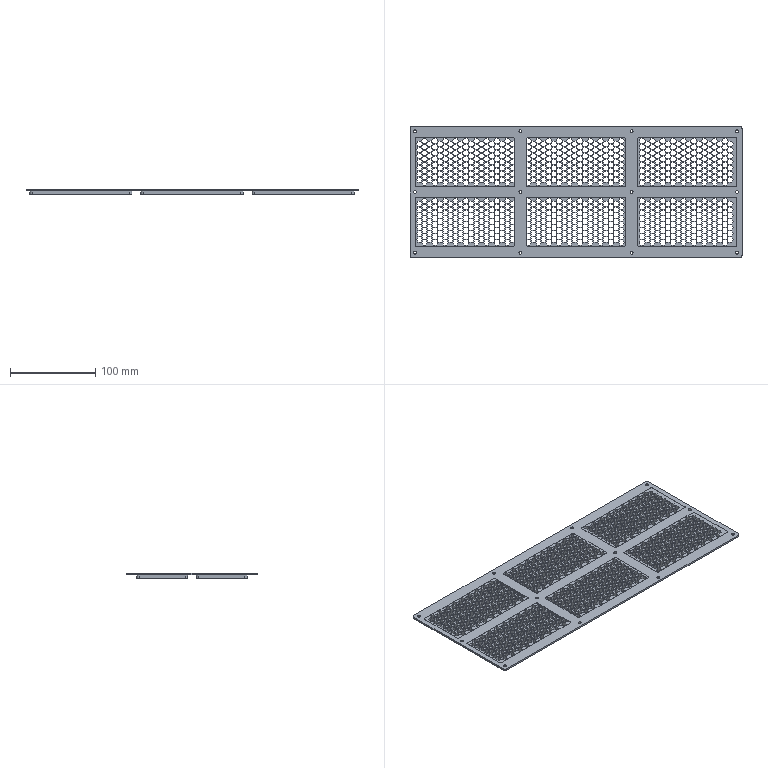NC program | NX | posted with a generic post
Lines 1 to 1112 of 172913:
N10 G17 G21 G94 G90
(PLANAR_MILL_3 , TOOL : D6_FINISH)
N12 T02 M6
N14 G54
N16 G17 G0 G90 X0. Y-79.75 S6500 M3
N18 G43 Z20. H2
N20 Z6.009
N22 G94 G1 Z3.009 F2000.
N24 Y-76.75
N26 X-191.5
N28 G2 X-194.25 Y-74. R2.75
N30 G1 Y74.
N32 G2 X-191.5 Y76.75 R2.75
N34 G1 X191.5
N36 G2 X194.25 Y74. R2.75
N38 G1 Y-74.
N40 G2 X191.5 Y-76.75 R2.75
N42 G1 X0.
N44 Y-71.95
N46 X-189.45
N48 Y-68.408
N50 G3 X-187. Y-68.86 R6.86
N52 G1 X-73.
N54 G3 X-66.659 Y-64.617 R6.86
N56 G1 X-62.222 Y-66.449
N58 G3 X-61.532 Y-67.15 R6.86
N60 G1 X-62.539
N62 X-65.437 Y-68.712
N64 X-62.539 Y-67.15
N66 G3 X-62.222 Y-66.449 R11.66
N68 G1 X-66.659 Y-64.617
N70 G3 X-66.14 Y-62. R6.86
N72 G1 Y-8.
N74 G3 X-73. Y-1.14 R6.86
N76 G1 X-187.
N78 G3 X-189.45 Y-1.592 R6.86
N80 G1 X-189.107 Y-2.489
N82 G2 X-187. Y-2.1 R5.9
N84 G1 X-73.
N86 G2 X-67.1 Y-8. R5.9
N88 G1 Y-62.
N90 G2 X-73. Y-67.9 R5.9
N92 G1 X-187.
N94 G2 X-192.9 Y-62. R5.9
N96 G1 Y-8.
N98 G2 X-189.107 Y-2.489 R5.9
N100 G1 X-189.45 Y-1.592
N102 Y1.592
N104 G3 X-187. Y1.14 R6.86
N106 G1 X-73.
N108 G3 X-66.14 Y8. R6.86
N110 G1 Y62.
N112 G3 X-73. Y68.86 R6.86
N114 G1 X-187.
N116 G3 X-189.45 Y68.408 R6.86
N118 G1 X-189.107 Y67.511
N120 G2 X-187. Y67.9 R5.9
N122 G1 X-73.
N124 G2 X-67.1 Y62. R5.9
N126 G1 Y8.
N128 G2 X-73. Y2.1 R5.9
N130 G1 X-187.
N132 G2 X-192.9 Y8. R5.9
N134 G1 Y62.
N136 G2 X-189.107 Y67.511 R5.9
N138 G1 X-189.45 Y68.408
N140 Y71.95
N142 X-61.532
N144 Y67.15
N146 G3 X-62.222 Y66.449 R6.86
N148 X-62.539 Y67.15 R11.66
N150 G1 X-65.437 Y68.712
N152 X-62.539 Y67.15
N154 X-61.532
N156 Y71.95
N158 X189.45
N160 Y68.408
N162 G3 X187. Y68.86 R6.86
N164 G1 X73.
N166 G3 X66.659 Y64.617 R6.86
N168 G1 X62.222 Y66.449
N170 G3 X61.532 Y67.15 R6.86
N172 G1 X59.132 Y68.95
N174 X-59.132
N176 G2 X-58.901 Y68.591 R3.
N178 X-57. Y68.86 R6.86
N180 G1 X57.
N182 G2 X58.901 Y68.591 R6.86
N184 X59.132 Y68.95 R3.
N186 G1 X61.532 Y67.15
N188 X62.539
N190 X65.437 Y68.712
N192 X62.539 Y67.15
N194 G3 X62.222 Y66.449 R11.66
N196 G1 X66.659 Y64.617
N198 G3 X66.14 Y62. R6.86
N200 G1 Y8.
N202 G3 X73. Y1.14 R6.86
N204 G1 X187.
N206 G3 X189.45 Y1.592 R6.86
N208 G1 X189.107 Y2.489
N210 G2 X187. Y2.1 R5.9
N212 G1 X73.
N214 G2 X67.1 Y8. R5.9
N216 G1 Y62.
N218 G2 X73. Y67.9 R5.9
N220 G1 X187.
N222 G2 X192.9 Y62. R5.9
N224 G1 Y8.
N226 G2 X189.107 Y2.489 R5.9
N228 G1 X189.45 Y1.592
N230 Y-1.592
N232 G3 X187. Y-1.14 R6.86
N234 G1 X73.
N236 G3 X66.659 Y-5.383 R6.86
N238 G1 X62.222 Y-3.551
N240 G3 X57. Y-1.14 R6.86
N242 G1 X-57.
N244 G3 X-62.222 Y-3.551 R6.86
N246 X-64.517 Y0. R11.66
N248 X-62.222 Y3.551 R11.66
N250 X-57. Y1.14 R6.86
N252 G1 X57.
N254 G3 X62.222 Y3.551 R6.86
N256 G1 X61.491 Y4.174
N258 G2 X57. Y2.1 R5.9
N260 G1 X-57.
N262 G2 X-62.9 Y8. R5.9
N264 G1 Y62.
N266 G2 X-57. Y67.9 R5.9
N268 G1 X57.
N270 G2 X62.9 Y62. R5.9
N272 G1 Y8.
N274 G2 X61.491 Y4.174 R5.9
N276 G1 X62.222 Y3.551
N278 G3 X64.517 Y0. R11.66
N280 X62.222 Y-3.551 R11.66
N282 G1 X66.659 Y-5.383
N284 G3 X66.14 Y-8. R6.86
N286 G1 Y-62.
N288 G3 X73. Y-68.86 R6.86
N290 G1 X187.
N292 G3 X189.45 Y-68.408 R6.86
N294 G1 X189.107 Y-67.511
N296 G2 X187. Y-67.9 R5.9
N298 G1 X73.
N300 G2 X67.1 Y-62. R5.9
N302 G1 Y-8.
N304 G2 X73. Y-2.1 R5.9
N306 G1 X187.
N308 G2 X192.9 Y-8. R5.9
N310 G1 Y-62.
N312 G2 X189.107 Y-67.511 R5.9
N314 G1 X189.45 Y-68.408
N316 Y-71.95
N318 X61.532
N320 Y-67.15
N322 G3 X62.222 Y-66.449 R6.86
N324 G1 X61.491 Y-65.826
N326 G2 X57. Y-67.9 R5.9
N328 G1 X-57.
N330 G2 X-62.9 Y-62. R5.9
N332 G1 Y-8.
N334 G2 X-57. Y-2.1 R5.9
N336 G1 X57.
N338 G2 X62.9 Y-8. R5.9
N340 G1 Y-62.
N342 G2 X61.491 Y-65.826 R5.9
N344 G1 X62.222 Y-66.449
N346 G3 X62.539 Y-67.15 R11.66
N348 G1 X65.437 Y-68.712
N350 X62.539 Y-67.15
N352 X61.532
N354 X58.901 Y-68.591
N356 G2 X57. Y-68.86 R6.86
N358 G1 X-57.
N360 G2 X-58.901 Y-68.591 R6.86
N362 X-59.132 Y-68.95 R3.
N364 G1 X59.132
N366 G2 X58.901 Y-68.591 R3.
N368 G1 X61.532 Y-67.15
N370 Y-71.95
N372 X0.
N374 Y-74.95
N376 Z6.009
N378 G0 Z20.
N380 Y-79.75
N382 Z5.519
N384 G1 Z2.519
N386 Y-76.75
N388 X-191.5
N390 G2 X-194.25 Y-74. R2.75
N392 G1 Y74.
N394 G2 X-191.5 Y76.75 R2.75
N396 G1 X191.5
N398 G2 X194.25 Y74. R2.75
N400 G1 Y-74.
N402 G2 X191.5 Y-76.75 R2.75
N404 G1 X0.
N406 Y-71.95
N408 X-189.45
N410 Y-68.408
N412 G3 X-187. Y-68.86 R6.86
N414 G1 X-73.
N416 G3 X-66.659 Y-64.617 R6.86
N418 G1 X-62.222 Y-66.449
N420 G3 X-61.532 Y-67.15 R6.86
N422 G1 X-62.539
N424 X-65.437 Y-68.712
N426 X-62.539 Y-67.15
N428 G3 X-62.222 Y-66.449 R11.66
N430 G1 X-66.659 Y-64.617
N432 G3 X-66.14 Y-62. R6.86
N434 G1 Y-8.
N436 G3 X-73. Y-1.14 R6.86
N438 G1 X-187.
N440 G3 X-189.45 Y-1.592 R6.86
N442 G1 X-189.107 Y-2.489
N444 G2 X-187. Y-2.1 R5.9
N446 G1 X-73.
N448 G2 X-67.1 Y-8. R5.9
N450 G1 Y-62.
N452 G2 X-73. Y-67.9 R5.9
N454 G1 X-187.
N456 G2 X-192.9 Y-62. R5.9
N458 G1 Y-8.
N460 G2 X-189.107 Y-2.489 R5.9
N462 G1 X-189.45 Y-1.592
N464 Y1.592
N466 G3 X-187. Y1.14 R6.86
N468 G1 X-73.
N470 G3 X-66.14 Y8. R6.86
N472 G1 Y62.
N474 G3 X-73. Y68.86 R6.86
N476 G1 X-187.
N478 G3 X-189.45 Y68.408 R6.86
N480 G1 X-189.107 Y67.511
N482 G2 X-187. Y67.9 R5.9
N484 G1 X-73.
N486 G2 X-67.1 Y62. R5.9
N488 G1 Y8.
N490 G2 X-73. Y2.1 R5.9
N492 G1 X-187.
N494 G2 X-192.9 Y8. R5.9
N496 G1 Y62.
N498 G2 X-189.107 Y67.511 R5.9
N500 G1 X-189.45 Y68.408
N502 Y71.95
N504 X-61.532
N506 Y67.15
N508 G3 X-62.222 Y66.449 R6.86
N510 X-62.539 Y67.15 R11.66
N512 G1 X-65.437 Y68.712
N514 X-62.539 Y67.15
N516 X-61.532
N518 Y71.95
N520 X189.45
N522 Y68.408
N524 G3 X187. Y68.86 R6.86
N526 G1 X73.
N528 G3 X66.659 Y64.617 R6.86
N530 G1 X62.222 Y66.449
N532 G3 X61.532 Y67.15 R6.86
N534 G1 X59.132 Y68.95
N536 X-59.132
N538 G2 X-58.901 Y68.591 R3.
N540 X-57. Y68.86 R6.86
N542 G1 X57.
N544 G2 X58.901 Y68.591 R6.86
N546 X59.132 Y68.95 R3.
N548 G1 X61.532 Y67.15
N550 X62.539
N552 X65.437 Y68.712
N554 X62.539 Y67.15
N556 G3 X62.222 Y66.449 R11.66
N558 G1 X66.659 Y64.617
N560 G3 X66.14 Y62. R6.86
N562 G1 Y8.
N564 G3 X73. Y1.14 R6.86
N566 G1 X187.
N568 G3 X189.45 Y1.592 R6.86
N570 G1 X189.107 Y2.489
N572 G2 X187. Y2.1 R5.9
N574 G1 X73.
N576 G2 X67.1 Y8. R5.9
N578 G1 Y62.
N580 G2 X73. Y67.9 R5.9
N582 G1 X187.
N584 G2 X192.9 Y62. R5.9
N586 G1 Y8.
N588 G2 X189.107 Y2.489 R5.9
N590 G1 X189.45 Y1.592
N592 Y-1.592
N594 G3 X187. Y-1.14 R6.86
N596 G1 X73.
N598 G3 X66.659 Y-5.383 R6.86
N600 G1 X62.222 Y-3.551
N602 G3 X57. Y-1.14 R6.86
N604 G1 X-57.
N606 G3 X-62.222 Y-3.551 R6.86
N608 X-64.517 Y0. R11.66
N610 X-62.222 Y3.551 R11.66
N612 X-57. Y1.14 R6.86
N614 G1 X57.
N616 G3 X62.222 Y3.551 R6.86
N618 G1 X61.491 Y4.174
N620 G2 X57. Y2.1 R5.9
N622 G1 X-57.
N624 G2 X-62.9 Y8. R5.9
N626 G1 Y62.
N628 G2 X-57. Y67.9 R5.9
N630 G1 X57.
N632 G2 X62.9 Y62. R5.9
N634 G1 Y8.
N636 G2 X61.491 Y4.174 R5.9
N638 G1 X62.222 Y3.551
N640 G3 X64.517 Y0. R11.66
N642 X62.222 Y-3.551 R11.66
N644 G1 X66.659 Y-5.383
N646 G3 X66.14 Y-8. R6.86
N648 G1 Y-62.
N650 G3 X73. Y-68.86 R6.86
N652 G1 X187.
N654 G3 X189.45 Y-68.408 R6.86
N656 G1 X189.107 Y-67.511
N658 G2 X187. Y-67.9 R5.9
N660 G1 X73.
N662 G2 X67.1 Y-62. R5.9
N664 G1 Y-8.
N666 G2 X73. Y-2.1 R5.9
N668 G1 X187.
N670 G2 X192.9 Y-8. R5.9
N672 G1 Y-62.
N674 G2 X189.107 Y-67.511 R5.9
N676 G1 X189.45 Y-68.408
N678 Y-71.95
N680 X61.532
N682 Y-67.15
N684 G3 X62.222 Y-66.449 R6.86
N686 G1 X61.491 Y-65.826
N688 G2 X57. Y-67.9 R5.9
N690 G1 X-57.
N692 G2 X-62.9 Y-62. R5.9
N694 G1 Y-8.
N696 G2 X-57. Y-2.1 R5.9
N698 G1 X57.
N700 G2 X62.9 Y-8. R5.9
N702 G1 Y-62.
N704 G2 X61.491 Y-65.826 R5.9
N706 G1 X62.222 Y-66.449
N708 G3 X62.539 Y-67.15 R11.66
N710 G1 X65.437 Y-68.712
N712 X62.539 Y-67.15
N714 X61.532
N716 X58.901 Y-68.591
N718 G2 X57. Y-68.86 R6.86
N720 G1 X-57.
N722 G2 X-58.901 Y-68.591 R6.86
N724 X-59.132 Y-68.95 R3.
N726 G1 X59.132
N728 G2 X58.901 Y-68.591 R3.
N730 G1 X61.532 Y-67.15
N732 Y-71.95
N734 X0.
N736 Y-74.95
N738 Z5.519
N740 G0 Z20.
N742 Y-79.75
N744 Z5.028
N746 G1 Z2.028
N748 Y-76.75
N750 X-191.5
N752 G2 X-194.25 Y-74. R2.75
N754 G1 Y74.
N756 G2 X-191.5 Y76.75 R2.75
N758 G1 X191.5
N760 G2 X194.25 Y74. R2.75
N762 G1 Y-74.
N764 G2 X191.5 Y-76.75 R2.75
N766 G1 X0.
N768 Y-71.95
N770 X-189.45
N772 Y-68.408
N774 G3 X-187. Y-68.86 R6.86
N776 G1 X-73.
N778 G3 X-66.659 Y-64.617 R6.86
N780 G1 X-62.222 Y-66.449
N782 G3 X-61.532 Y-67.15 R6.86
N784 G1 X-62.539
N786 X-65.437 Y-68.712
N788 X-62.539 Y-67.15
N790 G3 X-62.222 Y-66.449 R11.66
N792 G1 X-66.659 Y-64.617
N794 G3 X-66.14 Y-62. R6.86
N796 G1 Y-8.
N798 G3 X-73. Y-1.14 R6.86
N800 G1 X-187.
N802 G3 X-189.45 Y-1.592 R6.86
N804 G1 X-189.107 Y-2.489
N806 G2 X-187. Y-2.1 R5.9
N808 G1 X-73.
N810 G2 X-67.1 Y-8. R5.9
N812 G1 Y-62.
N814 G2 X-73. Y-67.9 R5.9
N816 G1 X-187.
N818 G2 X-192.9 Y-62. R5.9
N820 G1 Y-8.
N822 G2 X-189.107 Y-2.489 R5.9
N824 G1 X-189.45 Y-1.592
N826 Y1.592
N828 G3 X-187. Y1.14 R6.86
N830 G1 X-73.
N832 G3 X-66.14 Y8. R6.86
N834 G1 Y62.
N836 G3 X-73. Y68.86 R6.86
N838 G1 X-187.
N840 G3 X-189.45 Y68.408 R6.86
N842 G1 X-189.107 Y67.511
N844 G2 X-187. Y67.9 R5.9
N846 G1 X-73.
N848 G2 X-67.1 Y62. R5.9
N850 G1 Y8.
N852 G2 X-73. Y2.1 R5.9
N854 G1 X-187.
N856 G2 X-192.9 Y8. R5.9
N858 G1 Y62.
N860 G2 X-189.107 Y67.511 R5.9
N862 G1 X-189.45 Y68.408
N864 Y71.95
N866 X-61.532
N868 Y67.15
N870 G3 X-62.222 Y66.449 R6.86
N872 X-62.539 Y67.15 R11.66
N874 G1 X-65.437 Y68.712
N876 X-62.539 Y67.15
N878 X-61.532
N880 Y71.95
N882 X189.45
N884 Y68.408
N886 G3 X187. Y68.86 R6.86
N888 G1 X73.
N890 G3 X66.659 Y64.617 R6.86
N892 G1 X62.222 Y66.449
N894 G3 X61.532 Y67.15 R6.86
N896 G1 X59.132 Y68.95
N898 X-59.132
N900 G2 X-58.901 Y68.591 R3.
N902 X-57. Y68.86 R6.86
N904 G1 X57.
N906 G2 X58.901 Y68.591 R6.86
N908 X59.132 Y68.95 R3.
N910 G1 X61.532 Y67.15
N912 X62.539
N914 X65.437 Y68.712
N916 X62.539 Y67.15
N918 G3 X62.222 Y66.449 R11.66
N920 G1 X66.659 Y64.617
N922 G3 X66.14 Y62. R6.86
N924 G1 Y8.
N926 G3 X73. Y1.14 R6.86
N928 G1 X187.
N930 G3 X189.45 Y1.592 R6.86
N932 G1 X189.107 Y2.489
N934 G2 X187. Y2.1 R5.9
N936 G1 X73.
N938 G2 X67.1 Y8. R5.9
N940 G1 Y62.
N942 G2 X73. Y67.9 R5.9
N944 G1 X187.
N946 G2 X192.9 Y62. R5.9
N948 G1 Y8.
N950 G2 X189.107 Y2.489 R5.9
N952 G1 X189.45 Y1.592
N954 Y-1.592
N956 G3 X187. Y-1.14 R6.86
N958 G1 X73.
N960 G3 X66.659 Y-5.383 R6.86
N962 G1 X62.222 Y-3.551
N964 G3 X57. Y-1.14 R6.86
N966 G1 X-57.
N968 G3 X-62.222 Y-3.551 R6.86
N970 X-64.517 Y0. R11.66
N972 X-62.222 Y3.551 R11.66
N974 X-57. Y1.14 R6.86
N976 G1 X57.
N978 G3 X62.222 Y3.551 R6.86
N980 G1 X61.491 Y4.174
N982 G2 X57. Y2.1 R5.9
N984 G1 X-57.
N986 G2 X-62.9 Y8. R5.9
N988 G1 Y62.
N990 G2 X-57. Y67.9 R5.9
N992 G1 X57.
N994 G2 X62.9 Y62. R5.9
N996 G1 Y8.
N998 G2 X61.491 Y4.174 R5.9
N1000 G1 X62.222 Y3.551
N1002 G3 X64.517 Y0. R11.66
N1004 X62.222 Y-3.551 R11.66
N1006 G1 X66.659 Y-5.383
N1008 G3 X66.14 Y-8. R6.86
N1010 G1 Y-62.
N1012 G3 X73. Y-68.86 R6.86
N1014 G1 X187.
N1016 G3 X189.45 Y-68.408 R6.86
N1018 G1 X189.107 Y-67.511
N1020 G2 X187. Y-67.9 R5.9
N1022 G1 X73.
N1024 G2 X67.1 Y-62. R5.9
N1026 G1 Y-8.
N1028 G2 X73. Y-2.1 R5.9
N1030 G1 X187.
N1032 G2 X192.9 Y-8. R5.9
N1034 G1 Y-62.
N1036 G2 X189.107 Y-67.511 R5.9
N1038 G1 X189.45 Y-68.408
N1040 Y-71.95
N1042 X61.532
N1044 Y-67.15
N1046 G3 X62.222 Y-66.449 R6.86
N1048 G1 X61.491 Y-65.826
N1050 G2 X57. Y-67.9 R5.9
N1052 G1 X-57.
N1054 G2 X-62.9 Y-62. R5.9
N1056 G1 Y-8.
N1058 G2 X-57. Y-2.1 R5.9
N1060 G1 X57.
N1062 G2 X62.9 Y-8. R5.9
N1064 G1 Y-62.
N1066 G2 X61.491 Y-65.826 R5.9
N1068 G1 X62.222 Y-66.449
N1070 G3 X62.539 Y-67.15 R11.66
N1072 G1 X65.437 Y-68.712
N1074 X62.539 Y-67.15
N1076 X61.532
N1078 X58.901 Y-68.591
N1080 G2 X57. Y-68.86 R6.86
N1082 G1 X-57.
N1084 G2 X-58.901 Y-68.591 R6.86
N1086 X-59.132 Y-68.95 R3.
N1088 G1 X59.132
N1090 G2 X58.901 Y-68.591 R3.
N1092 G1 X61.532 Y-67.15
N1094 Y-71.95
N1096 X0.
N1098 Y-74.95
N1100 Z5.028
N1102 G0 Z20.
N1104 Y-79.75
N1106 Z4.538
N1108 G1 Z1.538
N1110 Y-76.75
N1112 X-191.5
N1114 G2 X-194.25 Y-74. R2.75
N1116 G1 Y74.
N1118 G2 X-191.5 Y76.75 R2.75
N1120 G1 X191.5
N1122 G2 X194.25 Y74. R2.75
N1124 G1 Y-74.
N1126 G2 X191.5 Y-76.75 R2.75
N1128 G1 X0.
N1130 Y-71.95
N1132 X-189.45
N1134 Y-68.408
N1136 G3 X-187. Y-68.86 R6.86
N1138 G1 X-73.
N1140 G3 X-66.659 Y-64.617 R6.86
N1142 G1 X-62.222 Y-66.449
N1144 G3 X-61.532 Y-67.15 R6.86
N1146 G1 X-62.539
N1148 X-65.437 Y-68.712
N1150 X-62.539 Y-67.15
N1152 G3 X-62.222 Y-66.449 R11.66
N1154 G1 X-66.659 Y-64.617
N1156 G3 X-66.14 Y-62. R6.86
N1158 G1 Y-8.
N1160 G3 X-73. Y-1.14 R6.86
N1162 G1 X-187.
N1164 G3 X-189.45 Y-1.592 R6.86
N1166 G1 X-189.107 Y-2.489
N1168 G2 X-187. Y-2.1 R5.9
N1170 G1 X-73.
N1172 G2 X-67.1 Y-8. R5.9
N1174 G1 Y-62.
N1176 G2 X-73. Y-67.9 R5.9
N1178 G1 X-187.
N1180 G2 X-192.9 Y-62. R5.9
N1182 G1 Y-8.
N1184 G2 X-189.107 Y-2.489 R5.9
N1186 G1 X-189.45 Y-1.592
N1188 Y1.592
N1190 G3 X-187. Y1.14 R6.86
N1192 G1 X-73.
N1194 G3 X-66.14 Y8. R6.86
N1196 G1 Y62.
N1198 G3 X-73. Y68.86 R6.86
N1200 G1 X-187.
N1202 G3 X-189.45 Y68.408 R6.86
N1204 G1 X-189.107 Y67.511
N1206 G2 X-187. Y67.9 R5.9
N1208 G1 X-73.
N1210 G2 X-67.1 Y62. R5.9
N1212 G1 Y8.
N1214 G2 X-73. Y2.1 R5.9
N1216 G1 X-187.
N1218 G2 X-192.9 Y8. R5.9
N1220 G1 Y62.
N1222 G2 X-189.107 Y67.511 R5.9
N1224 G1 X-189.45 Y68.408
N1226 Y71.95
N1228 X-61.532
N1230 Y67.15
N1232 G3 X-62.222 Y66.449 R6.86
N1234 X-62.539 Y67.15 R11.66
N1236 G1 X-65.437 Y68.712
N1238 X-62.539 Y67.15
N1240 X-61.532
N1242 Y71.95
N1244 X189.45
N1246 Y68.408
N1248 G3 X187. Y68.86 R6.86
N1250 G1 X73.
N1252 G3 X66.659 Y64.617 R6.86
N1254 G1 X62.222 Y66.449
N1256 G3 X61.532 Y67.15 R6.86
N1258 G1 X59.132 Y68.95
N1260 X-59.132
N1262 G2 X-58.901 Y68.591 R3.
N1264 X-57. Y68.86 R6.86
N1266 G1 X57.
N1268 G2 X58.901 Y68.591 R6.86
N1270 X59.132 Y68.95 R3.
N1272 G1 X61.532 Y67.15
N1274 X62.539
N1276 X65.437 Y68.712
N1278 X62.539 Y67.15
N1280 G3 X62.222 Y66.449 R11.66
N1282 G1 X66.659 Y64.617
N1284 G3 X66.14 Y62. R6.86
N1286 G1 Y8.
N1288 G3 X73. Y1.14 R6.86
N1290 G1 X187.
N1292 G3 X189.45 Y1.592 R6.86
N1294 G1 X189.107 Y2.489
N1296 G2 X187. Y2.1 R5.9
N1298 G1 X73.
N1300 G2 X67.1 Y8. R5.9
N1302 G1 Y62.
N1304 G2 X73. Y67.9 R5.9
N1306 G1 X187.
N1308 G2 X192.9 Y62. R5.9
N1310 G1 Y8.
N1312 G2 X189.107 Y2.489 R5.9
N1314 G1 X189.45 Y1.592
N1316 Y-1.592
N1318 G3 X187. Y-1.14 R6.86
N1320 G1 X73.
N1322 G3 X66.659 Y-5.383 R6.86
N1324 G1 X62.222 Y-3.551
N1326 G3 X57. Y-1.14 R6.86
N1328 G1 X-57.
N1330 G3 X-62.222 Y-3.551 R6.86
N1332 X-64.517 Y0. R11.66
N1334 X-62.222 Y3.551 R11.66
N1336 X-57. Y1.14 R6.86
N1338 G1 X57.
N1340 G3 X62.222 Y3.551 R6.86
N1342 G1 X61.491 Y4.174
N1344 G2 X57. Y2.1 R5.9
N1346 G1 X-57.
N1348 G2 X-62.9 Y8. R5.9
N1350 G1 Y62.
N1352 G2 X-57. Y67.9 R5.9
N1354 G1 X57.
N1356 G2 X62.9 Y62. R5.9
N1358 G1 Y8.
N1360 G2 X61.491 Y4.174 R5.9
N1362 G1 X62.222 Y3.551
N1364 G3 X64.517 Y0. R11.66
N1366 X62.222 Y-3.551 R11.66
N1368 G1 X66.659 Y-5.383
N1370 G3 X66.14 Y-8. R6.86
N1372 G1 Y-62.
N1374 G3 X73. Y-68.86 R6.86
N1376 G1 X187.
N1378 G3 X189.45 Y-68.408 R6.86
N1380 G1 X189.107 Y-67.511
N1382 G2 X187. Y-67.9 R5.9
N1384 G1 X73.
N1386 G2 X67.1 Y-62. R5.9
N1388 G1 Y-8.
N1390 G2 X73. Y-2.1 R5.9
N1392 G1 X187.
N1394 G2 X192.9 Y-8. R5.9
N1396 G1 Y-62.
N1398 G2 X189.107 Y-67.511 R5.9
N1400 G1 X189.45 Y-68.408
N1402 Y-71.95
N1404 X61.532
N1406 Y-67.15
N1408 G3 X62.222 Y-66.449 R6.86
N1410 G1 X61.491 Y-65.826
N1412 G2 X57. Y-67.9 R5.9
N1414 G1 X-57.
N1416 G2 X-62.9 Y-62. R5.9
N1418 G1 Y-8.
N1420 G2 X-57. Y-2.1 R5.9
N1422 G1 X57.
N1424 G2 X62.9 Y-8. R5.9
N1426 G1 Y-62.
N1428 G2 X61.491 Y-65.826 R5.9
N1430 G1 X62.222 Y-66.449
N1432 G3 X62.539 Y-67.15 R11.66
N1434 G1 X65.437 Y-68.712
N1436 X62.539 Y-67.15
N1438 X61.532
N1440 X58.901 Y-68.591
N1442 G2 X57. Y-68.86 R6.86
N1444 G1 X-57.
N1446 G2 X-58.901 Y-68.591 R6.86
N1448 X-59.132 Y-68.95 R3.
N1450 G1 X59.132
N1452 G2 X58.901 Y-68.591 R3.
N1454 G1 X61.532 Y-67.15
N1456 Y-71.95
N1458 X0.
N1460 Y-74.95
N1462 Z4.538
N1464 G0 Z20.
N1466 Y-79.75
N1468 Z4.047
N1470 G1 Z1.047
N1472 Y-76.75
N1474 X-191.5
N1476 G2 X-194.25 Y-74. R2.75
N1478 G1 Y74.
N1480 G2 X-191.5 Y76.75 R2.75
N1482 G1 X191.5
N1484 G2 X194.25 Y74. R2.75
N1486 G1 Y-74.
N1488 G2 X191.5 Y-76.75 R2.75
N1490 G1 X0.
N1492 Y-71.95
N1494 X-189.45
N1496 Y-68.408
N1498 G3 X-187. Y-68.86 R6.86
N1500 G1 X-73.
N1502 G3 X-66.659 Y-64.617 R6.86
N1504 G1 X-62.222 Y-66.449
N1506 G3 X-61.532 Y-67.15 R6.86
N1508 G1 X-62.539
N1510 X-65.437 Y-68.712
N1512 X-62.539 Y-67.15
N1514 G3 X-62.222 Y-66.449 R11.66
N1516 G1 X-66.659 Y-64.617
N1518 G3 X-66.14 Y-62. R6.86
N1520 G1 Y-8.
N1522 G3 X-73. Y-1.14 R6.86
N1524 G1 X-187.
N1526 G3 X-189.45 Y-1.592 R6.86
N1528 G1 X-189.107 Y-2.489
N1530 G2 X-187. Y-2.1 R5.9
N1532 G1 X-73.
N1534 G2 X-67.1 Y-8. R5.9
N1536 G1 Y-62.
N1538 G2 X-73. Y-67.9 R5.9
N1540 G1 X-187.
N1542 G2 X-192.9 Y-62. R5.9
N1544 G1 Y-8.
N1546 G2 X-189.107 Y-2.489 R5.9
N1548 G1 X-189.45 Y-1.592
N1550 Y1.592
N1552 G3 X-187. Y1.14 R6.86
N1554 G1 X-73.
N1556 G3 X-66.14 Y8. R6.86
N1558 G1 Y62.
N1560 G3 X-73. Y68.86 R6.86
N1562 G1 X-187.
N1564 G3 X-189.45 Y68.408 R6.86
N1566 G1 X-189.107 Y67.511
N1568 G2 X-187. Y67.9 R5.9
N1570 G1 X-73.
N1572 G2 X-67.1 Y62. R5.9
N1574 G1 Y8.
N1576 G2 X-73. Y2.1 R5.9
N1578 G1 X-187.
N1580 G2 X-192.9 Y8. R5.9
N1582 G1 Y62.
N1584 G2 X-189.107 Y67.511 R5.9
N1586 G1 X-189.45 Y68.408
N1588 Y71.95
N1590 X-61.532
N1592 Y67.15
N1594 G3 X-62.222 Y66.449 R6.86
N1596 X-62.539 Y67.15 R11.66
N1598 G1 X-65.437 Y68.712
N1600 X-62.539 Y67.15
N1602 X-61.532
N1604 Y71.95
N1606 X189.45
N1608 Y68.408
N1610 G3 X187. Y68.86 R6.86
N1612 G1 X73.
N1614 G3 X66.659 Y64.617 R6.86
N1616 G1 X62.222 Y66.449
N1618 G3 X61.532 Y67.15 R6.86
N1620 G1 X59.132 Y68.95
N1622 X-59.132
N1624 G2 X-58.901 Y68.591 R3.
N1626 X-57. Y68.86 R6.86
N1628 G1 X57.
N1630 G2 X58.901 Y68.591 R6.86
N1632 X59.132 Y68.95 R3.
N1634 G1 X61.532 Y67.15
N1636 X62.539
N1638 X65.437 Y68.712
N1640 X62.539 Y67.15
N1642 G3 X62.222 Y66.449 R11.66
N1644 G1 X66.659 Y64.617
N1646 G3 X66.14 Y62. R6.86
N1648 G1 Y8.
N1650 G3 X73. Y1.14 R6.86
N1652 G1 X187.
N1654 G3 X189.45 Y1.592 R6.86
N1656 G1 X189.107 Y2.489
N1658 G2 X187. Y2.1 R5.9
N1660 G1 X73.
N1662 G2 X67.1 Y8. R5.9
N1664 G1 Y62.
N1666 G2 X73. Y67.9 R5.9
N1668 G1 X187.
N1670 G2 X192.9 Y62. R5.9
N1672 G1 Y8.
N1674 G2 X189.107 Y2.489 R5.9
N1676 G1 X189.45 Y1.592
N1678 Y-1.592
N1680 G3 X187. Y-1.14 R6.86
N1682 G1 X73.
N1684 G3 X66.659 Y-5.383 R6.86
N1686 G1 X62.222 Y-3.551
N1688 G3 X57. Y-1.14 R6.86
N1690 G1 X-57.
N1692 G3 X-62.222 Y-3.551 R6.86
N1694 X-64.517 Y0. R11.66
N1696 X-62.222 Y3.551 R11.66
N1698 X-57. Y1.14 R6.86
N1700 G1 X57.
N1702 G3 X62.222 Y3.551 R6.86
N1704 G1 X61.491 Y4.174
N1706 G2 X57. Y2.1 R5.9
N1708 G1 X-57.
N1710 G2 X-62.9 Y8. R5.9
N1712 G1 Y62.
N1714 G2 X-57. Y67.9 R5.9
N1716 G1 X57.
N1718 G2 X62.9 Y62. R5.9
N1720 G1 Y8.
N1722 G2 X61.491 Y4.174 R5.9
N1724 G1 X62.222 Y3.551
N1726 G3 X64.517 Y0. R11.66
N1728 X62.222 Y-3.551 R11.66
N1730 G1 X66.659 Y-5.383
N1732 G3 X66.14 Y-8. R6.86
N1734 G1 Y-62.
N1736 G3 X73. Y-68.86 R6.86
N1738 G1 X187.
N1740 G3 X189.45 Y-68.408 R6.86
N1742 G1 X189.107 Y-67.511
N1744 G2 X187. Y-67.9 R5.9
N1746 G1 X73.
N1748 G2 X67.1 Y-62. R5.9
N1750 G1 Y-8.
N1752 G2 X73. Y-2.1 R5.9
N1754 G1 X187.
N1756 G2 X192.9 Y-8. R5.9
N1758 G1 Y-62.
N1760 G2 X189.107 Y-67.511 R5.9
N1762 G1 X189.45 Y-68.408
N1764 Y-71.95
N1766 X61.532
N1768 Y-67.15
N1770 G3 X62.222 Y-66.449 R6.86
N1772 G1 X61.491 Y-65.826
N1774 G2 X57. Y-67.9 R5.9
N1776 G1 X-57.
N1778 G2 X-62.9 Y-62. R5.9
N1780 G1 Y-8.
N1782 G2 X-57. Y-2.1 R5.9
N1784 G1 X57.
N1786 G2 X62.9 Y-8. R5.9
N1788 G1 Y-62.
N1790 G2 X61.491 Y-65.826 R5.9
N1792 G1 X62.222 Y-66.449
N1794 G3 X62.539 Y-67.15 R11.66
N1796 G1 X65.437 Y-68.712
N1798 X62.539 Y-67.15
N1800 X61.532
N1802 X58.901 Y-68.591
N1804 G2 X57. Y-68.86 R6.86
N1806 G1 X-57.
N1808 G2 X-58.901 Y-68.591 R6.86
N1810 X-59.132 Y-68.95 R3.
N1812 G1 X59.132
N1814 G2 X58.901 Y-68.591 R3.
N1816 G1 X61.532 Y-67.15
N1818 Y-71.95
N1820 X0.
N1822 Y-74.95
N1824 Z4.047
N1826 G0 Z20.
N1828 Y-79.75
N1830 Z3.556
N1832 G1 Z0.556
N1834 Y-76.75
N1836 X-191.5
N1838 G2 X-194.25 Y-74. R2.75
N1840 G1 Y74.
N1842 G2 X-191.5 Y76.75 R2.75
N1844 G1 X191.5
N1846 G2 X194.25 Y74. R2.75
N1848 G1 Y-74.
N1850 G2 X191.5 Y-76.75 R2.75
N1852 G1 X0.
N1854 Y-71.95
N1856 X-189.45
N1858 Y-68.408
N1860 G3 X-187. Y-68.86 R6.86
N1862 G1 X-73.
N1864 G3 X-66.659 Y-64.617 R6.86
N1866 G1 X-62.222 Y-66.449
N1868 G3 X-61.532 Y-67.15 R6.86
N1870 G1 X-62.539
N1872 X-65.437 Y-68.712
N1874 X-62.539 Y-67.15
N1876 G3 X-62.222 Y-66.449 R11.66
N1878 G1 X-66.659 Y-64.617
N1880 G3 X-66.14 Y-62. R6.86
N1882 G1 Y-8.
N1884 G3 X-73. Y-1.14 R6.86
N1886 G1 X-187.
N1888 G3 X-189.45 Y-1.592 R6.86
N1890 G1 X-189.107 Y-2.489
N1892 G2 X-187. Y-2.1 R5.9
N1894 G1 X-73.
N1896 G2 X-67.1 Y-8. R5.9
N1898 G1 Y-62.
N1900 G2 X-73. Y-67.9 R5.9
N1902 G1 X-187.
N1904 G2 X-192.9 Y-62. R5.9
N1906 G1 Y-8.
N1908 G2 X-189.107 Y-2.489 R5.9
N1910 G1 X-189.45 Y-1.592
N1912 Y1.592
N1914 G3 X-187. Y1.14 R6.86
N1916 G1 X-73.
N1918 G3 X-66.14 Y8. R6.86
N1920 G1 Y62.
N1922 G3 X-73. Y68.86 R6.86
N1924 G1 X-187.
N1926 G3 X-189.45 Y68.408 R6.86
N1928 G1 X-189.107 Y67.511
N1930 G2 X-187. Y67.9 R5.9
N1932 G1 X-73.
N1934 G2 X-67.1 Y62. R5.9
N1936 G1 Y8.
N1938 G2 X-73. Y2.1 R5.9
N1940 G1 X-187.
N1942 G2 X-192.9 Y8. R5.9
N1944 G1 Y62.
N1946 G2 X-189.107 Y67.511 R5.9
N1948 G1 X-189.45 Y68.408
N1950 Y71.95
N1952 X-61.532
N1954 Y67.15
N1956 G3 X-62.222 Y66.449 R6.86
N1958 X-62.539 Y67.15 R11.66
N1960 G1 X-65.437 Y68.712
N1962 X-62.539 Y67.15
N1964 X-61.532
N1966 Y71.95
N1968 X189.45
N1970 Y68.408
N1972 G3 X187. Y68.86 R6.86
N1974 G1 X73.
N1976 G3 X66.659 Y64.617 R6.86
N1978 G1 X62.222 Y66.449
N1980 G3 X61.532 Y67.15 R6.86
N1982 G1 X59.132 Y68.95
N1984 X-59.132
N1986 G2 X-58.901 Y68.591 R3.
N1988 X-57. Y68.86 R6.86
N1990 G1 X57.
N1992 G2 X58.901 Y68.591 R6.86
N1994 X59.132 Y68.95 R3.
N1996 G1 X61.532 Y67.15
N1998 X62.539
N2000 X65.437 Y68.712
N2002 X62.539 Y67.15
N2004 G3 X62.222 Y66.449 R11.66
N2006 G1 X66.659 Y64.617
N2008 G3 X66.14 Y62. R6.86
N2010 G1 Y8.
N2012 G3 X73. Y1.14 R6.86
N2014 G1 X187.
N2016 G3 X189.45 Y1.592 R6.86
N2018 G1 X189.107 Y2.489
N2020 G2 X187. Y2.1 R5.9
N2022 G1 X73.
N2024 G2 X67.1 Y8. R5.9
N2026 G1 Y62.
N2028 G2 X73. Y67.9 R5.9
N2030 G1 X187.
N2032 G2 X192.9 Y62. R5.9
N2034 G1 Y8.
N2036 G2 X189.107 Y2.489 R5.9
N2038 G1 X189.45 Y1.592
N2040 Y-1.592
N2042 G3 X187. Y-1.14 R6.86
N2044 G1 X73.
N2046 G3 X66.659 Y-5.383 R6.86
N2048 G1 X62.222 Y-3.551
N2050 G3 X57. Y-1.14 R6.86
N2052 G1 X-57.
N2054 G3 X-62.222 Y-3.551 R6.86
N2056 X-64.517 Y0. R11.66
N2058 X-62.222 Y3.551 R11.66
N2060 X-57. Y1.14 R6.86
N2062 G1 X57.
N2064 G3 X62.222 Y3.551 R6.86
N2066 G1 X61.491 Y4.174
N2068 G2 X57. Y2.1 R5.9
N2070 G1 X-57.
N2072 G2 X-62.9 Y8. R5.9
N2074 G1 Y62.
N2076 G2 X-57. Y67.9 R5.9
N2078 G1 X57.
N2080 G2 X62.9 Y62. R5.9
N2082 G1 Y8.
N2084 G2 X61.491 Y4.174 R5.9
N2086 G1 X62.222 Y3.551
N2088 G3 X64.517 Y0. R11.66
N2090 X62.222 Y-3.551 R11.66
N2092 G1 X66.659 Y-5.383
N2094 G3 X66.14 Y-8. R6.86
N2096 G1 Y-62.
N2098 G3 X73. Y-68.86 R6.86
N2100 G1 X187.
N2102 G3 X189.45 Y-68.408 R6.86
N2104 G1 X189.107 Y-67.511
N2106 G2 X187. Y-67.9 R5.9
N2108 G1 X73.
N2110 G2 X67.1 Y-62. R5.9
N2112 G1 Y-8.
N2114 G2 X73. Y-2.1 R5.9
N2116 G1 X187.
N2118 G2 X192.9 Y-8. R5.9
N2120 G1 Y-62.
N2122 G2 X189.107 Y-67.511 R5.9
N2124 G1 X189.45 Y-68.408
N2126 Y-71.95
N2128 X61.532
N2130 Y-67.15
N2132 G3 X62.222 Y-66.449 R6.86
N2134 G1 X61.491 Y-65.826
N2136 G2 X57. Y-67.9 R5.9
N2138 G1 X-57.
N2140 G2 X-62.9 Y-62. R5.9
N2142 G1 Y-8.
N2144 G2 X-57. Y-2.1 R5.9
N2146 G1 X57.
N2148 G2 X62.9 Y-8. R5.9
N2150 G1 Y-62.
N2152 G2 X61.491 Y-65.826 R5.9
N2154 G1 X62.222 Y-66.449
N2156 G3 X62.539 Y-67.15 R11.66
N2158 G1 X65.437 Y-68.712
N2160 X62.539 Y-67.15
N2162 X61.532
N2164 X58.901 Y-68.591
N2166 G2 X57. Y-68.86 R6.86
N2168 G1 X-57.
N2170 G2 X-58.901 Y-68.591 R6.86
N2172 X-59.132 Y-68.95 R3.
N2174 G1 X59.132
N2176 G2 X58.901 Y-68.591 R3.
N2178 G1 X61.532 Y-67.15
N2180 Y-71.95
N2182 X0.
N2184 Y-74.95
N2186 Z3.556
N2188 G0 Z20.
N2190 Y-79.75
N2192 Z3.066
N2194 G1 Z0.066
N2196 Y-76.75
N2198 X-191.5
N2200 G2 X-194.25 Y-74. R2.75
N2202 G1 Y74.
N2204 G2 X-191.5 Y76.75 R2.75
N2206 G1 X191.5
N2208 G2 X194.25 Y74. R2.75
N2210 G1 Y-74.
N2212 G2 X191.5 Y-76.75 R2.75
N2214 G1 X0.
N2216 Y-71.95
N2218 X-189.45
N2220 Y-68.408
N2222 G3 X-187. Y-68.86 R6.86